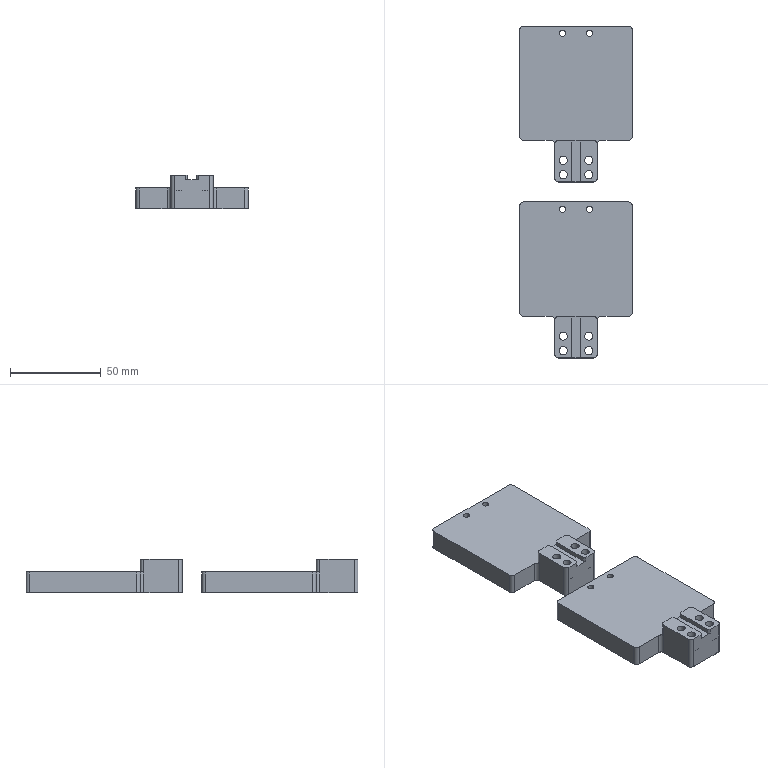Part | 2 solids | 124 faces | box 62 x 183 x 18.5 mm | volume 103167 mm3 | cylinder 68 | plane 48 | cone 8 | commonest cylinder face diameters 4 x20 3.3 x16 4.5 x16 7.9 x16